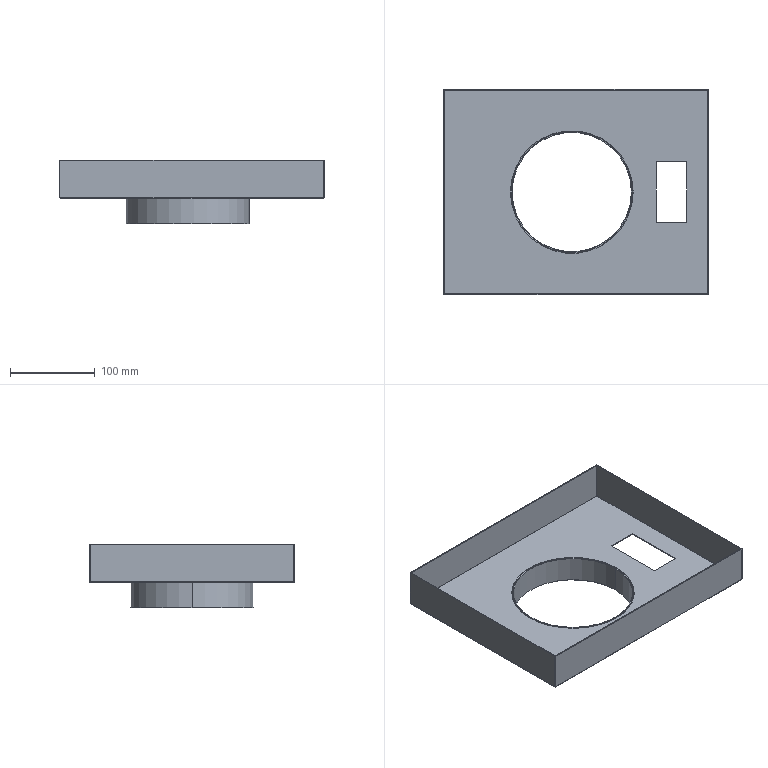Part | STEP file | RJWD-DY-01010001 | 2 solids | 58 faces | box 312.4 x 242.4 x 75 mm | volume 132718 mm3 | plane 32 | cylinder 16 | spline 8 | torus 2 | commonest cylinder face diameters 0.4 x4 2.4 x4 143 x4 141 x2 145 x2